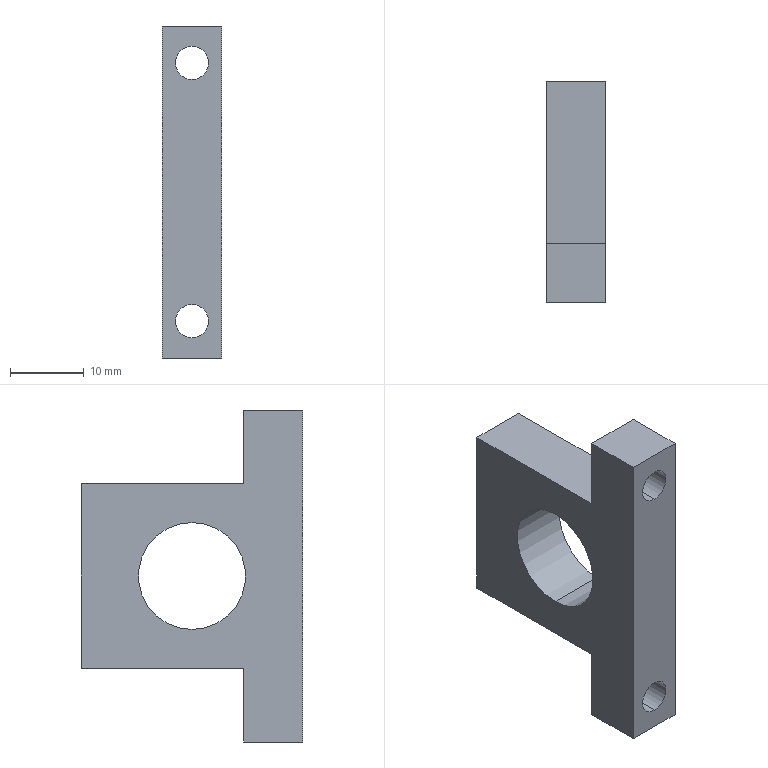Part | STEP file | 04-09 Suction rotary cylinder fixing plate | 1 solid | 16 faces | box 8 x 30 x 45 mm | volume 5704 mm3 | plane 10 | cylinder 6 | commonest cylinder face diameters 4.5 x4 14.5 x2
STEP:
#1=CARTESIAN_POINT('',(0.,0.,0.));
#2=DIRECTION('',(0.,0.,1.));
#3=DIRECTION('',(1.,0.,0.));
#4=AXIS2_PLACEMENT_3D('',#1,#2,#3);
#5=CARTESIAN_POINT('',(4.,0.,19.75));
#6=VERTEX_POINT('',#5);
#7=CARTESIAN_POINT('',(4.,8.,19.75));
#8=VERTEX_POINT('',#7);
#9=CARTESIAN_POINT('',(4.,0.,19.75));
#10=DIRECTION('',(0.,1.,0.));
#11=VECTOR('',#10,1.);
#12=LINE('',#9,#11);
#13=CARTESIAN_POINT('',(4.,0.,17.5));
#14=DIRECTION('',(0.,1.,0.));
#15=DIRECTION('',(0.,0.,1.));
#16=AXIS2_PLACEMENT_3D('',#13,#14,#15);
#17=CYLINDRICAL_SURFACE('',#16,2.25);
#18=CARTESIAN_POINT('',(6.283,0.));
#19=DIRECTION('',(0.,1.));
#20=VECTOR('',#19,1.);
#21=LINE('',#18,#20);
#22=(GEOMETRIC_REPRESENTATION_CONTEXT(2)PARAMETRIC_REPRESENTATION_CONTEXT()REPRESENTATION_CONTEXT('',''));
#23=DEFINITIONAL_REPRESENTATION('',(#21),#22);
#24=PCURVE('',#17,#23);
#25=CARTESIAN_POINT('',(4.,0.,17.5));
#26=DIRECTION('',(0.,1.,0.));
#27=DIRECTION('',(0.,0.,1.));
#28=AXIS2_PLACEMENT_3D('',#25,#26,#27);
#29=CYLINDRICAL_SURFACE('',#28,2.25);
#30=CARTESIAN_POINT('',(0.,0.));
#31=DIRECTION('',(0.,1.));
#32=VECTOR('',#31,1.);
#33=LINE('',#30,#32);
#34=(GEOMETRIC_REPRESENTATION_CONTEXT(2)PARAMETRIC_REPRESENTATION_CONTEXT()REPRESENTATION_CONTEXT('',''));
#35=DEFINITIONAL_REPRESENTATION('',(#33),#34);
#36=PCURVE('',#29,#35);
#37=SURFACE_CURVE('',#12,(#24,#36),.PCURVE_S1.);
#38=EDGE_CURVE('',#6,#8,#37,.T.);
#39=ORIENTED_EDGE('',*,*,#38,.T.);
#40=CARTESIAN_POINT('',(4.,8.,15.25));
#41=VERTEX_POINT('',#40);
#42=CARTESIAN_POINT('',(4.,8.,17.5));
#43=DIRECTION('',(0.,1.,0.));
#44=DIRECTION('',(0.,0.,1.));
#45=AXIS2_PLACEMENT_3D('',#42,#43,#44);
#46=CIRCLE('',#45,2.25);
#47=CARTESIAN_POINT('',(0.,8.));
#48=DIRECTION('',(1.,0.));
#49=VECTOR('',#48,1.);
#50=LINE('',#47,#49);
#51=(GEOMETRIC_REPRESENTATION_CONTEXT(2)PARAMETRIC_REPRESENTATION_CONTEXT()REPRESENTATION_CONTEXT('',''));
#52=DEFINITIONAL_REPRESENTATION('',(#50),#51);
#53=PCURVE('',#17,#52);
#54=CARTESIAN_POINT('',(0.,8.,22.5));
#55=DIRECTION('',(0.,-1.,0.));
#56=DIRECTION('',(0.,0.,-1.));
#57=AXIS2_PLACEMENT_3D('',#54,#55,#56);
#58=PLANE('',#57);
#59=CARTESIAN_POINT('',(2.75,4.));
#60=CARTESIAN_POINT('',(2.75,7.897));
#61=CARTESIAN_POINT('',(6.125,5.949));
#62=CARTESIAN_POINT('',(9.5,4.));
#63=CARTESIAN_POINT('',(6.125,2.051));
#64=CARTESIAN_POINT('',(2.75,0.1029));
#65=CARTESIAN_POINT('',(2.75,4.));
#66=(BOUNDED_CURVE()B_SPLINE_CURVE(2,(#59,#60,#61,#62,#63,#64,#65),.UNSPECIFIED.,.T.,.F.)B_SPLINE_CURVE_WITH_KNOTS((1,2,2,2,2,1),(-2.094,0.,2.094,4.189,6.283,8.378),.UNSPECIFIED.)CURVE()GEOMETRIC_REPRESENTATION_ITEM()RATIONAL_B_SPLINE_CURVE((1.,0.5,1.,0.5,1.,0.5,1.))REPRESENTATION_ITEM(''));
#67=(GEOMETRIC_REPRESENTATION_CONTEXT(2)PARAMETRIC_REPRESENTATION_CONTEXT()REPRESENTATION_CONTEXT('',''));
#68=DEFINITIONAL_REPRESENTATION('',(#66),#67);
#69=PCURVE('',#58,#68);
#70=SURFACE_CURVE('',#46,(#53,#69),.PCURVE_S1.);
#71=EDGE_CURVE('',#41,#8,#70,.T.);
#72=ORIENTED_EDGE('',*,*,#71,.F.);
#73=CARTESIAN_POINT('',(4.,0.,15.25));
#74=VERTEX_POINT('',#73);
#75=CARTESIAN_POINT('',(4.,0.,15.25));
#76=DIRECTION('',(0.,1.,0.));
#77=VECTOR('',#76,1.);
#78=LINE('',#75,#77);
#79=CARTESIAN_POINT('',(3.142,0.));
#80=DIRECTION('',(0.,1.));
#81=VECTOR('',#80,1.);
#82=LINE('',#79,#81);
#83=(GEOMETRIC_REPRESENTATION_CONTEXT(2)PARAMETRIC_REPRESENTATION_CONTEXT()REPRESENTATION_CONTEXT('',''));
#84=DEFINITIONAL_REPRESENTATION('',(#82),#83);
#85=PCURVE('',#17,#84);
#86=CARTESIAN_POINT('',(3.142,0.));
#87=DIRECTION('',(0.,1.));
#88=VECTOR('',#87,1.);
#89=LINE('',#86,#88);
#90=(GEOMETRIC_REPRESENTATION_CONTEXT(2)PARAMETRIC_REPRESENTATION_CONTEXT()REPRESENTATION_CONTEXT('',''));
#91=DEFINITIONAL_REPRESENTATION('',(#89),#90);
#92=PCURVE('',#29,#91);
#93=SURFACE_CURVE('',#78,(#85,#92),.PCURVE_S1.);
#94=EDGE_CURVE('',#74,#41,#93,.T.);
#95=ORIENTED_EDGE('',*,*,#94,.F.);
#96=CARTESIAN_POINT('',(4.,0.,17.5));
#97=DIRECTION('',(0.,-1.,0.));
#98=DIRECTION('',(0.,0.,1.));
#99=AXIS2_PLACEMENT_3D('',#96,#97,#98);
#100=CIRCLE('',#99,2.25);
#101=CARTESIAN_POINT('',(6.283,0.));
#102=DIRECTION('',(-1.,0.));
#103=VECTOR('',#102,1.);
#104=LINE('',#101,#103);
#105=(GEOMETRIC_REPRESENTATION_CONTEXT(2)PARAMETRIC_REPRESENTATION_CONTEXT()REPRESENTATION_CONTEXT('',''));
#106=DEFINITIONAL_REPRESENTATION('',(#104),#105);
#107=PCURVE('',#17,#106);
#108=CARTESIAN_POINT('',(0.,0.,-22.5));
#109=DIRECTION('',(0.,1.,0.));
#110=DIRECTION('',(0.,0.,1.));
#111=AXIS2_PLACEMENT_3D('',#108,#109,#110);
#112=PLANE('',#111);
#113=CARTESIAN_POINT('',(42.25,4.));
#114=CARTESIAN_POINT('',(42.25,0.1029));
#115=CARTESIAN_POINT('',(38.875,2.051));
#116=CARTESIAN_POINT('',(35.5,4.));
#117=CARTESIAN_POINT('',(38.875,5.949));
#118=CARTESIAN_POINT('',(42.25,7.897));
#119=CARTESIAN_POINT('',(42.25,4.));
#120=(BOUNDED_CURVE()B_SPLINE_CURVE(2,(#113,#114,#115,#116,#117,#118,#119),.UNSPECIFIED.,.T.,.F.)B_SPLINE_CURVE_WITH_KNOTS((1,2,2,2,2,1),(-2.094,0.,2.094,4.189,6.283,8.378),.UNSPECIFIED.)CURVE()GEOMETRIC_REPRESENTATION_ITEM()RATIONAL_B_SPLINE_CURVE((1.,0.5,1.,0.5,1.,0.5,1.))REPRESENTATION_ITEM(''));
#121=(GEOMETRIC_REPRESENTATION_CONTEXT(2)PARAMETRIC_REPRESENTATION_CONTEXT()REPRESENTATION_CONTEXT('',''));
#122=DEFINITIONAL_REPRESENTATION('',(#120),#121);
#123=PCURVE('',#112,#122);
#124=SURFACE_CURVE('',#100,(#107,#123),.PCURVE_S1.);
#125=EDGE_CURVE('',#6,#74,#124,.T.);
#126=ORIENTED_EDGE('',*,*,#125,.F.);
#127=EDGE_LOOP('',(#39,#72,#95,#126));
#128=FACE_BOUND('',#127,.F.);
#129=ADVANCED_FACE('',(#128),#17,.F.);
#130=CARTESIAN_POINT('',(4.,0.,-15.25));
#131=VERTEX_POINT('',#130);
#132=CARTESIAN_POINT('',(4.,8.,-15.25));
#133=VERTEX_POINT('',#132);
#134=CARTESIAN_POINT('',(4.,0.,-15.25));
#135=DIRECTION('',(0.,1.,0.));
#136=VECTOR('',#135,1.);
#137=LINE('',#134,#136);
#138=CARTESIAN_POINT('',(4.,0.,-17.5));
#139=DIRECTION('',(0.,1.,0.));
#140=DIRECTION('',(0.,0.,1.));
#141=AXIS2_PLACEMENT_3D('',#138,#139,#140);
#142=CYLINDRICAL_SURFACE('',#141,2.25);
#143=CARTESIAN_POINT('',(6.283,0.));
#144=DIRECTION('',(0.,1.));
#145=VECTOR('',#144,1.);
#146=LINE('',#143,#145);
#147=(GEOMETRIC_REPRESENTATION_CONTEXT(2)PARAMETRIC_REPRESENTATION_CONTEXT()REPRESENTATION_CONTEXT('',''));
#148=DEFINITIONAL_REPRESENTATION('',(#146),#147);
#149=PCURVE('',#142,#148);
#150=CARTESIAN_POINT('',(4.,0.,-17.5));
#151=DIRECTION('',(0.,1.,0.));
#152=DIRECTION('',(0.,0.,1.));
#153=AXIS2_PLACEMENT_3D('',#150,#151,#152);
#154=CYLINDRICAL_SURFACE('',#153,2.25);
#155=CARTESIAN_POINT('',(0.,0.));
#156=DIRECTION('',(0.,1.));
#157=VECTOR('',#156,1.);
#158=LINE('',#155,#157);
#159=(GEOMETRIC_REPRESENTATION_CONTEXT(2)PARAMETRIC_REPRESENTATION_CONTEXT()REPRESENTATION_CONTEXT('',''));
#160=DEFINITIONAL_REPRESENTATION('',(#158),#159);
#161=PCURVE('',#154,#160);
#162=SURFACE_CURVE('',#137,(#149,#161),.PCURVE_S1.);
#163=EDGE_CURVE('',#131,#133,#162,.T.);
#164=ORIENTED_EDGE('',*,*,#163,.T.);
#165=CARTESIAN_POINT('',(4.,8.,-19.75));
#166=VERTEX_POINT('',#165);
#167=CARTESIAN_POINT('',(4.,8.,-17.5));
#168=DIRECTION('',(0.,1.,0.));
#169=DIRECTION('',(0.,0.,1.));
#170=AXIS2_PLACEMENT_3D('',#167,#168,#169);
#171=CIRCLE('',#170,2.25);
#172=CARTESIAN_POINT('',(0.,8.));
#173=DIRECTION('',(1.,0.));
#174=VECTOR('',#173,1.);
#175=LINE('',#172,#174);
#176=(GEOMETRIC_REPRESENTATION_CONTEXT(2)PARAMETRIC_REPRESENTATION_CONTEXT()REPRESENTATION_CONTEXT('',''));
#177=DEFINITIONAL_REPRESENTATION('',(#175),#176);
#178=PCURVE('',#142,#177);
#179=CARTESIAN_POINT('',(0.,8.,-12.5));
#180=DIRECTION('',(0.,-1.,0.));
#181=DIRECTION('',(0.,0.,-1.));
#182=AXIS2_PLACEMENT_3D('',#179,#180,#181);
#183=PLANE('',#182);
#184=CARTESIAN_POINT('',(2.75,4.));
#185=CARTESIAN_POINT('',(2.75,7.897));
#186=CARTESIAN_POINT('',(6.125,5.949));
#187=CARTESIAN_POINT('',(9.5,4.));
#188=CARTESIAN_POINT('',(6.125,2.051));
#189=CARTESIAN_POINT('',(2.75,0.1029));
#190=CARTESIAN_POINT('',(2.75,4.));
#191=(BOUNDED_CURVE()B_SPLINE_CURVE(2,(#184,#185,#186,#187,#188,#189,#190),.UNSPECIFIED.,.T.,.F.)B_SPLINE_CURVE_WITH_KNOTS((1,2,2,2,2,1),(-2.094,0.,2.094,4.189,6.283,8.378),.UNSPECIFIED.)CURVE()GEOMETRIC_REPRESENTATION_ITEM()RATIONAL_B_SPLINE_CURVE((1.,0.5,1.,0.5,1.,0.5,1.))REPRESENTATION_ITEM(''));
#192=(GEOMETRIC_REPRESENTATION_CONTEXT(2)PARAMETRIC_REPRESENTATION_CONTEXT()REPRESENTATION_CONTEXT('',''));
#193=DEFINITIONAL_REPRESENTATION('',(#191),#192);
#194=PCURVE('',#183,#193);
#195=SURFACE_CURVE('',#171,(#178,#194),.PCURVE_S1.);
#196=EDGE_CURVE('',#166,#133,#195,.T.);
#197=ORIENTED_EDGE('',*,*,#196,.F.);
#198=CARTESIAN_POINT('',(4.,0.,-19.75));
#199=VERTEX_POINT('',#198);
#200=CARTESIAN_POINT('',(4.,0.,-19.75));
#201=DIRECTION('',(0.,1.,0.));
#202=VECTOR('',#201,1.);
#203=LINE('',#200,#202);
#204=CARTESIAN_POINT('',(3.142,0.));
#205=DIRECTION('',(0.,1.));
#206=VECTOR('',#205,1.);
#207=LINE('',#204,#206);
#208=(GEOMETRIC_REPRESENTATION_CONTEXT(2)PARAMETRIC_REPRESENTATION_CONTEXT()REPRESENTATION_CONTEXT('',''));
#209=DEFINITIONAL_REPRESENTATION('',(#207),#208);
#210=PCURVE('',#142,#209);
#211=CARTESIAN_POINT('',(3.142,0.));
#212=DIRECTION('',(0.,1.));
#213=VECTOR('',#212,1.);
#214=LINE('',#211,#213);
#215=(GEOMETRIC_REPRESENTATION_CONTEXT(2)PARAMETRIC_REPRESENTATION_CONTEXT()REPRESENTATION_CONTEXT('',''));
#216=DEFINITIONAL_REPRESENTATION('',(#214),#215);
#217=PCURVE('',#154,#216);
#218=SURFACE_CURVE('',#203,(#210,#217),.PCURVE_S1.);
#219=EDGE_CURVE('',#199,#166,#218,.T.);
#220=ORIENTED_EDGE('',*,*,#219,.F.);
#221=CARTESIAN_POINT('',(4.,0.,-17.5));
#222=DIRECTION('',(0.,-1.,0.));
#223=DIRECTION('',(0.,0.,1.));
#224=AXIS2_PLACEMENT_3D('',#221,#222,#223);
#225=CIRCLE('',#224,2.25);
#226=CARTESIAN_POINT('',(6.283,0.));
#227=DIRECTION('',(-1.,0.));
#228=VECTOR('',#227,1.);
#229=LINE('',#226,#228);
#230=(GEOMETRIC_REPRESENTATION_CONTEXT(2)PARAMETRIC_REPRESENTATION_CONTEXT()REPRESENTATION_CONTEXT('',''));
#231=DEFINITIONAL_REPRESENTATION('',(#229),#230);
#232=PCURVE('',#142,#231);
#233=CARTESIAN_POINT('',(7.25,4.));
#234=CARTESIAN_POINT('',(7.25,0.1029));
#235=CARTESIAN_POINT('',(3.875,2.051));
#236=CARTESIAN_POINT('',(0.5,4.));
#237=CARTESIAN_POINT('',(3.875,5.949));
#238=CARTESIAN_POINT('',(7.25,7.897));
#239=CARTESIAN_POINT('',(7.25,4.));
#240=(BOUNDED_CURVE()B_SPLINE_CURVE(2,(#233,#234,#235,#236,#237,#238,#239),.UNSPECIFIED.,.T.,.F.)B_SPLINE_CURVE_WITH_KNOTS((1,2,2,2,2,1),(-2.094,0.,2.094,4.189,6.283,8.378),.UNSPECIFIED.)CURVE()GEOMETRIC_REPRESENTATION_ITEM()RATIONAL_B_SPLINE_CURVE((1.,0.5,1.,0.5,1.,0.5,1.))REPRESENTATION_ITEM(''));
#241=(GEOMETRIC_REPRESENTATION_CONTEXT(2)PARAMETRIC_REPRESENTATION_CONTEXT()REPRESENTATION_CONTEXT('',''));
#242=DEFINITIONAL_REPRESENTATION('',(#240),#241);
#243=PCURVE('',#112,#242);
#244=SURFACE_CURVE('',#225,(#232,#243),.PCURVE_S1.);
#245=EDGE_CURVE('',#131,#199,#244,.T.);
#246=ORIENTED_EDGE('',*,*,#245,.F.);
#247=EDGE_LOOP('',(#164,#197,#220,#246));
#248=FACE_BOUND('',#247,.F.);
#249=ADVANCED_FACE('',(#248),#142,.F.);
#250=CARTESIAN_POINT('',(0.,15.,-7.25));
#251=VERTEX_POINT('',#250);
#252=CARTESIAN_POINT('',(8.,15.,-7.25));
#253=VERTEX_POINT('',#252);
#254=CARTESIAN_POINT('',(0.,15.,-7.25));
#255=DIRECTION('',(1.,0.,0.));
#256=VECTOR('',#255,1.);
#257=LINE('',#254,#256);
#258=CARTESIAN_POINT('',(0.,15.,0.));
#259=DIRECTION('',(1.,0.,0.));
#260=DIRECTION('',(0.,0.,-1.));
#261=AXIS2_PLACEMENT_3D('',#258,#259,#260);
#262=CYLINDRICAL_SURFACE('',#261,7.25);
#263=CARTESIAN_POINT('',(6.283,0.));
#264=DIRECTION('',(0.,1.));
#265=VECTOR('',#264,1.);
#266=LINE('',#263,#265);
#267=(GEOMETRIC_REPRESENTATION_CONTEXT(2)PARAMETRIC_REPRESENTATION_CONTEXT()REPRESENTATION_CONTEXT('',''));
#268=DEFINITIONAL_REPRESENTATION('',(#266),#267);
#269=PCURVE('',#262,#268);
#270=CARTESIAN_POINT('',(0.,15.,0.));
#271=DIRECTION('',(1.,0.,0.));
#272=DIRECTION('',(0.,0.,-1.));
#273=AXIS2_PLACEMENT_3D('',#270,#271,#272);
#274=CYLINDRICAL_SURFACE('',#273,7.25);
#275=CARTESIAN_POINT('',(0.,0.));
#276=DIRECTION('',(0.,1.));
#277=VECTOR('',#276,1.);
#278=LINE('',#275,#277);
#279=(GEOMETRIC_REPRESENTATION_CONTEXT(2)PARAMETRIC_REPRESENTATION_CONTEXT()REPRESENTATION_CONTEXT('',''));
#280=DEFINITIONAL_REPRESENTATION('',(#278),#279);
#281=PCURVE('',#274,#280);
#282=SURFACE_CURVE('',#257,(#269,#281),.PCURVE_S1.);
#283=EDGE_CURVE('',#251,#253,#282,.T.);
#284=ORIENTED_EDGE('',*,*,#283,.T.);
#285=CARTESIAN_POINT('',(8.,15.,7.25));
#286=VERTEX_POINT('',#285);
#287=CARTESIAN_POINT('',(8.,15.,0.));
#288=DIRECTION('',(1.,0.,0.));
#289=DIRECTION('',(0.,0.,-1.));
#290=AXIS2_PLACEMENT_3D('',#287,#288,#289);
#291=CIRCLE('',#290,7.25);
#292=CARTESIAN_POINT('',(0.,8.));
#293=DIRECTION('',(1.,0.));
#294=VECTOR('',#293,1.);
#295=LINE('',#292,#294);
#296=(GEOMETRIC_REPRESENTATION_CONTEXT(2)PARAMETRIC_REPRESENTATION_CONTEXT()REPRESENTATION_CONTEXT('',''));
#297=DEFINITIONAL_REPRESENTATION('',(#295),#296);
#298=PCURVE('',#262,#297);
#299=CARTESIAN_POINT('',(8.,0.,-22.5));
#300=DIRECTION('',(-1.,0.,0.));
#301=DIRECTION('',(0.,0.,1.));
#302=AXIS2_PLACEMENT_3D('',#299,#300,#301);
#303=PLANE('',#302);
#304=CARTESIAN_POINT('',(15.25,15.));
#305=CARTESIAN_POINT('',(15.25,27.557));
#306=CARTESIAN_POINT('',(26.125,21.279));
#307=CARTESIAN_POINT('',(37.,15.));
#308=CARTESIAN_POINT('',(26.125,8.721));
#309=CARTESIAN_POINT('',(15.25,2.443));
#310=CARTESIAN_POINT('',(15.25,15.));
#311=(BOUNDED_CURVE()B_SPLINE_CURVE(2,(#304,#305,#306,#307,#308,#309,#310),.UNSPECIFIED.,.T.,.F.)B_SPLINE_CURVE_WITH_KNOTS((1,2,2,2,2,1),(-2.094,0.,2.094,4.189,6.283,8.378),.UNSPECIFIED.)CURVE()GEOMETRIC_REPRESENTATION_ITEM()RATIONAL_B_SPLINE_CURVE((1.,0.5,1.,0.5,1.,0.5,1.))REPRESENTATION_ITEM(''));
#312=(GEOMETRIC_REPRESENTATION_CONTEXT(2)PARAMETRIC_REPRESENTATION_CONTEXT()REPRESENTATION_CONTEXT('',''));
#313=DEFINITIONAL_REPRESENTATION('',(#311),#312);
#314=PCURVE('',#303,#313);
#315=SURFACE_CURVE('',#291,(#298,#314),.PCURVE_S1.);
#316=EDGE_CURVE('',#286,#253,#315,.T.);
#317=ORIENTED_EDGE('',*,*,#316,.F.);
#318=CARTESIAN_POINT('',(0.,15.,7.25));
#319=VERTEX_POINT('',#318);
#320=CARTESIAN_POINT('',(0.,15.,7.25));
#321=DIRECTION('',(1.,0.,0.));
#322=VECTOR('',#321,1.);
#323=LINE('',#320,#322);
#324=CARTESIAN_POINT('',(3.142,0.));
#325=DIRECTION('',(0.,1.));
#326=VECTOR('',#325,1.);
#327=LINE('',#324,#326);
#328=(GEOMETRIC_REPRESENTATION_CONTEXT(2)PARAMETRIC_REPRESENTATION_CONTEXT()REPRESENTATION_CONTEXT('',''));
#329=DEFINITIONAL_REPRESENTATION('',(#327),#328);
#330=PCURVE('',#262,#329);
#331=CARTESIAN_POINT('',(3.142,0.));
#332=DIRECTION('',(0.,1.));
#333=VECTOR('',#332,1.);
#334=LINE('',#331,#333);
#335=(GEOMETRIC_REPRESENTATION_CONTEXT(2)PARAMETRIC_REPRESENTATION_CONTEXT()REPRESENTATION_CONTEXT('',''));
#336=DEFINITIONAL_REPRESENTATION('',(#334),#335);
#337=PCURVE('',#274,#336);
#338=SURFACE_CURVE('',#323,(#330,#337),.PCURVE_S1.);
#339=EDGE_CURVE('',#319,#286,#338,.T.);
#340=ORIENTED_EDGE('',*,*,#339,.F.);
#341=CARTESIAN_POINT('',(0.,15.,0.));
#342=DIRECTION('',(1.,0.,0.));
#343=DIRECTION('',(0.,0.,-1.));
#344=AXIS2_PLACEMENT_3D('',#341,#342,#343);
#345=CIRCLE('',#344,7.25);
#346=CARTESIAN_POINT('',(0.,0.));
#347=DIRECTION('',(1.,0.));
#348=VECTOR('',#347,1.);
#349=LINE('',#346,#348);
#350=(GEOMETRIC_REPRESENTATION_CONTEXT(2)PARAMETRIC_REPRESENTATION_CONTEXT()REPRESENTATION_CONTEXT('',''));
#351=DEFINITIONAL_REPRESENTATION('',(#349),#350);
#352=PCURVE('',#262,#351);
#353=CARTESIAN_POINT('',(0.,0.,-22.5));
#354=DIRECTION('',(-1.,0.,0.));
#355=DIRECTION('',(0.,0.,1.));
#356=AXIS2_PLACEMENT_3D('',#353,#354,#355);
#357=PLANE('',#356);
#358=CARTESIAN_POINT('',(15.25,15.));
#359=CARTESIAN_POINT('',(15.25,27.557));
#360=CARTESIAN_POINT('',(26.125,21.279));
#361=CARTESIAN_POINT('',(37.,15.));
#362=CARTESIAN_POINT('',(26.125,8.721));
#363=CARTESIAN_POINT('',(15.25,2.443));
#364=CARTESIAN_POINT('',(15.25,15.));
#365=(BOUNDED_CURVE()B_SPLINE_CURVE(2,(#358,#359,#360,#361,#362,#363,#364),.UNSPECIFIED.,.T.,.F.)B_SPLINE_CURVE_WITH_KNOTS((1,2,2,2,2,1),(-2.094,0.,2.094,4.189,6.283,8.378),.UNSPECIFIED.)CURVE()GEOMETRIC_REPRESENTATION_ITEM()RATIONAL_B_SPLINE_CURVE((1.,0.5,1.,0.5,1.,0.5,1.))REPRESENTATION_ITEM(''));
#366=(GEOMETRIC_REPRESENTATION_CONTEXT(2)PARAMETRIC_REPRESENTATION_CONTEXT()REPRESENTATION_CONTEXT('',''));
#367=DEFINITIONAL_REPRESENTATION('',(#365),#366);
#368=PCURVE('',#357,#367);
#369=SURFACE_CURVE('',#345,(#352,#368),.PCURVE_S1.);
#370=EDGE_CURVE('',#319,#251,#369,.T.);
#371=ORIENTED_EDGE('',*,*,#370,.T.);
#372=EDGE_LOOP('',(#284,#317,#340,#371));
#373=FACE_BOUND('',#372,.F.);
#374=ADVANCED_FACE('',(#373),#262,.F.);
#375=CARTESIAN_POINT('',(4.,8.,17.5));
#376=DIRECTION('',(0.,1.,0.));
#377=DIRECTION('',(0.,0.,1.));
#378=AXIS2_PLACEMENT_3D('',#375,#376,#377);
#379=CIRCLE('',#378,2.25);
#380=CARTESIAN_POINT('',(0.,8.));
#381=DIRECTION('',(1.,0.));
#382=VECTOR('',#381,1.);
#383=LINE('',#380,#382);
#384=(GEOMETRIC_REPRESENTATION_CONTEXT(2)PARAMETRIC_REPRESENTATION_CONTEXT()REPRESENTATION_CONTEXT('',''));
#385=DEFINITIONAL_REPRESENTATION('',(#383),#384);
#386=PCURVE('',#29,#385);
#387=CARTESIAN_POINT('',(2.75,4.));
#388=CARTESIAN_POINT('',(2.75,7.897));
#389=CARTESIAN_POINT('',(6.125,5.949));
#390=CARTESIAN_POINT('',(9.5,4.));
#391=CARTESIAN_POINT('',(6.125,2.051));
#392=CARTESIAN_POINT('',(2.75,0.1029));
#393=CARTESIAN_POINT('',(2.75,4.));
#394=(BOUNDED_CURVE()B_SPLINE_CURVE(2,(#387,#388,#389,#390,#391,#392,#393),.UNSPECIFIED.,.T.,.F.)B_SPLINE_CURVE_WITH_KNOTS((1,2,2,2,2,1),(-2.094,0.,2.094,4.189,6.283,8.378),.UNSPECIFIED.)CURVE()GEOMETRIC_REPRESENTATION_ITEM()RATIONAL_B_SPLINE_CURVE((1.,0.5,1.,0.5,1.,0.5,1.))REPRESENTATION_ITEM(''));
#395=(GEOMETRIC_REPRESENTATION_CONTEXT(2)PARAMETRIC_REPRESENTATION_CONTEXT()REPRESENTATION_CONTEXT('',''));
#396=DEFINITIONAL_REPRESENTATION('',(#394),#395);
#397=PCURVE('',#58,#396);
#398=SURFACE_CURVE('',#379,(#386,#397),.PCURVE_S1.);
#399=EDGE_CURVE('',#8,#41,#398,.T.);
#400=ORIENTED_EDGE('',*,*,#399,.F.);
#401=ORIENTED_EDGE('',*,*,#38,.F.);
#402=CARTESIAN_POINT('',(4.,0.,17.5));
#403=DIRECTION('',(0.,-1.,0.));
#404=DIRECTION('',(0.,0.,1.));
#405=AXIS2_PLACEMENT_3D('',#402,#403,#404);
#406=CIRCLE('',#405,2.25);
#407=CARTESIAN_POINT('',(6.283,0.));
#408=DIRECTION('',(-1.,0.));
#409=VECTOR('',#408,1.);
#410=LINE('',#407,#409);
#411=(GEOMETRIC_REPRESENTATION_CONTEXT(2)PARAMETRIC_REPRESENTATION_CONTEXT()REPRESENTATION_CONTEXT('',''));
#412=DEFINITIONAL_REPRESENTATION('',(#410),#411);
#413=PCURVE('',#29,#412);
#414=CARTESIAN_POINT('',(42.25,4.));
#415=CARTESIAN_POINT('',(42.25,0.1029));
#416=CARTESIAN_POINT('',(38.875,2.051));
#417=CARTESIAN_POINT('',(35.5,4.));
#418=CARTESIAN_POINT('',(38.875,5.949));
#419=CARTESIAN_POINT('',(42.25,7.897));
#420=CARTESIAN_POINT('',(42.25,4.));
#421=(BOUNDED_CURVE()B_SPLINE_CURVE(2,(#414,#415,#416,#417,#418,#419,#420),.UNSPECIFIED.,.T.,.F.)B_SPLINE_CURVE_WITH_KNOTS((1,2,2,2,2,1),(-2.094,0.,2.094,4.189,6.283,8.378),.UNSPECIFIED.)CURVE()GEOMETRIC_REPRESENTATION_ITEM()RATIONAL_B_SPLINE_CURVE((1.,0.5,1.,0.5,1.,0.5,1.))REPRESENTATION_ITEM(''));
#422=(GEOMETRIC_REPRESENTATION_CONTEXT(2)PARAMETRIC_REPRESENTATION_CONTEXT()REPRESENTATION_CONTEXT('',''));
#423=DEFINITIONAL_REPRESENTATION('',(#421),#422);
#424=PCURVE('',#112,#423);
#425=SURFACE_CURVE('',#406,(#413,#424),.PCURVE_S1.);
#426=EDGE_CURVE('',#74,#6,#425,.T.);
#427=ORIENTED_EDGE('',*,*,#426,.F.);
#428=ORIENTED_EDGE('',*,*,#94,.T.);
#429=EDGE_LOOP('',(#400,#401,#427,#428));
#430=FACE_BOUND('',#429,.F.);
#431=ADVANCED_FACE('',(#430),#29,.F.);
#432=ORIENTED_EDGE('',*,*,#399,.F.);
#433=ORIENTED_EDGE('',*,*,#71,.F.);
#434=EDGE_LOOP('',(#432,#433));
#435=FACE_BOUND('',#434,.T.);
#436=CARTESIAN_POINT('',(8.,8.,22.5));
#437=VERTEX_POINT('',#436);
#438=CARTESIAN_POINT('',(0.,8.,22.5));
#439=VERTEX_POINT('',#438);
#440=CARTESIAN_POINT('',(4.,8.,22.5));
#441=DIRECTION('',(-1.,0.,0.));
#442=VECTOR('',#441,1.);
#443=LINE('',#440,#442);
#444=CARTESIAN_POINT('',(0.,4.));
#445=DIRECTION('',(0.,-1.));
#446=VECTOR('',#445,1.);
#447=LINE('',#444,#446);
#448=(GEOMETRIC_REPRESENTATION_CONTEXT(2)PARAMETRIC_REPRESENTATION_CONTEXT()REPRESENTATION_CONTEXT('',''));
#449=DEFINITIONAL_REPRESENTATION('',(#447),#448);
#450=PCURVE('',#58,#449);
#451=CARTESIAN_POINT('',(8.,0.,22.5));
#452=DIRECTION('',(0.,0.,-1.));
#453=DIRECTION('',(-1.,0.,0.));
#454=AXIS2_PLACEMENT_3D('',#451,#452,#453);
#455=PLANE('',#454);
#456=CARTESIAN_POINT('',(4.,8.));
#457=DIRECTION('',(1.,0.));
#458=VECTOR('',#457,1.);
#459=LINE('',#456,#458);
#460=(GEOMETRIC_REPRESENTATION_CONTEXT(2)PARAMETRIC_REPRESENTATION_CONTEXT()REPRESENTATION_CONTEXT('',''));
#461=DEFINITIONAL_REPRESENTATION('',(#459),#460);
#462=PCURVE('',#455,#461);
#463=SURFACE_CURVE('',#443,(#450,#462),.PCURVE_S1.);
#464=EDGE_CURVE('',#437,#439,#463,.T.);
#465=ORIENTED_EDGE('',*,*,#464,.F.);
#466=CARTESIAN_POINT('',(8.,8.,12.5));
#467=VERTEX_POINT('',#466);
#468=CARTESIAN_POINT('',(8.,8.,17.5));
#469=DIRECTION('',(0.,0.,1.));
#470=VECTOR('',#469,1.);
#471=LINE('',#468,#470);
#472=CARTESIAN_POINT('',(5.,8.));
#473=DIRECTION('',(-1.,0.));
#474=VECTOR('',#473,1.);
#475=LINE('',#472,#474);
#476=(GEOMETRIC_REPRESENTATION_CONTEXT(2)PARAMETRIC_REPRESENTATION_CONTEXT()REPRESENTATION_CONTEXT('',''));
#477=DEFINITIONAL_REPRESENTATION('',(#475),#476);
#478=PCURVE('',#58,#477);
#479=CARTESIAN_POINT('',(40.,8.));
#480=DIRECTION('',(1.,0.));
#481=VECTOR('',#480,1.);
#482=LINE('',#479,#481);
#483=(GEOMETRIC_REPRESENTATION_CONTEXT(2)PARAMETRIC_REPRESENTATION_CONTEXT()REPRESENTATION_CONTEXT('',''));
#484=DEFINITIONAL_REPRESENTATION('',(#482),#483);
#485=PCURVE('',#303,#484);
#486=SURFACE_CURVE('',#471,(#478,#485),.PCURVE_S1.);
#487=EDGE_CURVE('',#467,#437,#486,.T.);
#488=ORIENTED_EDGE('',*,*,#487,.F.);
#489=CARTESIAN_POINT('',(0.,8.,12.5));
#490=VERTEX_POINT('',#489);
#491=CARTESIAN_POINT('',(4.,8.,12.5));
#492=DIRECTION('',(1.,0.,0.));
#493=VECTOR('',#492,1.);
#494=LINE('',#491,#493);
#495=CARTESIAN_POINT('',(10.,4.));
#496=DIRECTION('',(0.,1.));
#497=VECTOR('',#496,1.);
#498=LINE('',#495,#497);
#499=(GEOMETRIC_REPRESENTATION_CONTEXT(2)PARAMETRIC_REPRESENTATION_CONTEXT()REPRESENTATION_CONTEXT('',''));
#500=DEFINITIONAL_REPRESENTATION('',(#498),#499);
#501=PCURVE('',#58,#500);
#502=CARTESIAN_POINT('',(0.,8.,12.5));
#503=DIRECTION('',(0.,0.,-1.));
#504=DIRECTION('',(0.,1.,0.));
#505=AXIS2_PLACEMENT_3D('',#502,#503,#504);
#506=PLANE('',#505);
#507=CARTESIAN_POINT('',(0.,4.));
#508=DIRECTION('',(0.,1.));
#509=VECTOR('',#508,1.);
#510=LINE('',#507,#509);
#511=(GEOMETRIC_REPRESENTATION_CONTEXT(2)PARAMETRIC_REPRESENTATION_CONTEXT()REPRESENTATION_CONTEXT('',''));
#512=DEFINITIONAL_REPRESENTATION('',(#510),#511);
#513=PCURVE('',#506,#512);
#514=SURFACE_CURVE('',#494,(#501,#513),.PCURVE_S1.);
#515=EDGE_CURVE('',#490,#467,#514,.T.);
#516=ORIENTED_EDGE('',*,*,#515,.F.);
#517=CARTESIAN_POINT('',(0.,8.,17.5));
#518=DIRECTION('',(0.,0.,-1.));
#519=VECTOR('',#518,1.);
#520=LINE('',#517,#519);
#521=CARTESIAN_POINT('',(5.,0.));
#522=DIRECTION('',(1.,0.));
#523=VECTOR('',#522,1.);
#524=LINE('',#521,#523);
#525=(GEOMETRIC_REPRESENTATION_CONTEXT(2)PARAMETRIC_REPRESENTATION_CONTEXT()REPRESENTATION_CONTEXT('',''));
#526=DEFINITIONAL_REPRESENTATION('',(#524),#525);
#527=PCURVE('',#58,#526);
#528=CARTESIAN_POINT('',(40.,8.));
#529=DIRECTION('',(-1.,0.));
#530=VECTOR('',#529,1.);
#531=LINE('',#528,#530);
#532=(GEOMETRIC_REPRESENTATION_CONTEXT(2)PARAMETRIC_REPRESENTATION_CONTEXT()REPRESENTATION_CONTEXT('',''));
#533=DEFINITIONAL_REPRESENTATION('',(#531),#532);
#534=PCURVE('',#357,#533);
#535=SURFACE_CURVE('',#520,(#527,#534),.PCURVE_S1.);
#536=EDGE_CURVE('',#439,#490,#535,.T.);
#537=ORIENTED_EDGE('',*,*,#536,.F.);
#538=EDGE_LOOP('',(#465,#488,#516,#537));
#539=FACE_BOUND('',#538,.T.);
#540=ADVANCED_FACE('',(#435,#539),#58,.F.);
#541=ORIENTED_EDGE('',*,*,#245,.F.);
#542=CARTESIAN_POINT('',(4.,0.,-17.5));
#543=DIRECTION('',(0.,-1.,0.));
#544=DIRECTION('',(0.,0.,1.));
#545=AXIS2_PLACEMENT_3D('',#542,#543,#544);
#546=CIRCLE('',#545,2.25);
#547=CARTESIAN_POINT('',(7.25,4.));
#548=CARTESIAN_POINT('',(7.25,0.1029));
#549=CARTESIAN_POINT('',(3.875,2.051));
#550=CARTESIAN_POINT('',(0.5,4.));
#551=CARTESIAN_POINT('',(3.875,5.949));
#552=CARTESIAN_POINT('',(7.25,7.897));
#553=CARTESIAN_POINT('',(7.25,4.));
#554=(BOUNDED_CURVE()B_SPLINE_CURVE(2,(#547,#548,#549,#550,#551,#552,#553),.UNSPECIFIED.,.T.,.F.)B_SPLINE_CURVE_WITH_KNOTS((1,2,2,2,2,1),(-2.094,0.,2.094,4.189,6.283,8.378),.UNSPECIFIED.)CURVE()GEOMETRIC_REPRESENTATION_ITEM()RATIONAL_B_SPLINE_CURVE((1.,0.5,1.,0.5,1.,0.5,1.))REPRESENTATION_ITEM(''));
#555=(GEOMETRIC_REPRESENTATION_CONTEXT(2)PARAMETRIC_REPRESENTATION_CONTEXT()REPRESENTATION_CONTEXT('',''));
#556=DEFINITIONAL_REPRESENTATION('',(#554),#555);
#557=PCURVE('',#112,#556);
#558=CARTESIAN_POINT('',(6.283,0.));
#559=DIRECTION('',(-1.,0.));
#560=VECTOR('',#559,1.);
#561=LINE('',#558,#560);
#562=(GEOMETRIC_REPRESENTATION_CONTEXT(2)PARAMETRIC_REPRESENTATION_CONTEXT()REPRESENTATION_CONTEXT('',''));
#563=DEFINITIONAL_REPRESENTATION('',(#561),#562);
#564=PCURVE('',#154,#563);
#565=SURFACE_CURVE('',#546,(#557,#564),.PCURVE_S1.);
#566=EDGE_CURVE('',#199,#131,#565,.T.);
#567=ORIENTED_EDGE('',*,*,#566,.F.);
#568=EDGE_LOOP('',(#541,#567));
#569=FACE_BOUND('',#568,.T.);
#570=ORIENTED_EDGE('',*,*,#125,.F.);
#571=ORIENTED_EDGE('',*,*,#426,.F.);
#572=EDGE_LOOP('',(#570,#571));
#573=FACE_BOUND('',#572,.T.);
#574=CARTESIAN_POINT('',(8.,0.,-22.5));
#575=VERTEX_POINT('',#574);
#576=CARTESIAN_POINT('',(0.,0.,-22.5));
#577=VERTEX_POINT('',#576);
#578=CARTESIAN_POINT('',(4.,0.,-22.5));
#579=DIRECTION('',(-1.,0.,0.));
#580=VECTOR('',#579,1.);
#581=LINE('',#578,#580);
#582=CARTESIAN_POINT('',(0.,4.));
#583=DIRECTION('',(0.,-1.));
#584=VECTOR('',#583,1.);
#585=LINE('',#582,#584);
#586=(GEOMETRIC_REPRESENTATION_CONTEXT(2)PARAMETRIC_REPRESENTATION_CONTEXT()REPRESENTATION_CONTEXT('',''));
#587=DEFINITIONAL_REPRESENTATION('',(#585),#586);
#588=PCURVE('',#112,#587);
#589=CARTESIAN_POINT('',(0.,0.,-22.5));
#590=DIRECTION('',(0.,0.,1.));
#591=DIRECTION('',(1.,0.,0.));
#592=AXIS2_PLACEMENT_3D('',#589,#590,#591);
#593=PLANE('',#592);
#594=CARTESIAN_POINT('',(4.,0.));
#595=DIRECTION('',(-1.,0.));
#596=VECTOR('',#595,1.);
#597=LINE('',#594,#596);
#598=(GEOMETRIC_REPRESENTATION_CONTEXT(2)PARAMETRIC_REPRESENTATION_CONTEXT()REPRESENTATION_CONTEXT('',''));
#599=DEFINITIONAL_REPRESENTATION('',(#597),#598);
#600=PCURVE('',#593,#599);
#601=SURFACE_CURVE('',#581,(#588,#600),.PCURVE_S1.);
#602=EDGE_CURVE('',#575,#577,#601,.T.);
#603=ORIENTED_EDGE('',*,*,#602,.F.);
#604=CARTESIAN_POINT('',(8.,0.,22.5));
#605=VERTEX_POINT('',#604);
#606=CARTESIAN_POINT('',(8.,0.,0.));
#607=DIRECTION('',(0.,0.,-1.));
#608=VECTOR('',#607,1.);
#609=LINE('',#606,#608);
#610=CARTESIAN_POINT('',(22.5,8.));
#611=DIRECTION('',(-1.,0.));
#612=VECTOR('',#611,1.);
#613=LINE('',#610,#612);
#614=(GEOMETRIC_REPRESENTATION_CONTEXT(2)PARAMETRIC_REPRESENTATION_CONTEXT()REPRESENTATION_CONTEXT('',''));
#615=DEFINITIONAL_REPRESENTATION('',(#613),#614);
#616=PCURVE('',#112,#615);
#617=CARTESIAN_POINT('',(22.5,0.));
#618=DIRECTION('',(-1.,0.));
#619=VECTOR('',#618,1.);
#620=LINE('',#617,#619);
#621=(GEOMETRIC_REPRESENTATION_CONTEXT(2)PARAMETRIC_REPRESENTATION_CONTEXT()REPRESENTATION_CONTEXT('',''));
#622=DEFINITIONAL_REPRESENTATION('',(#620),#621);
#623=PCURVE('',#303,#622);
#624=SURFACE_CURVE('',#609,(#616,#623),.PCURVE_S1.);
#625=EDGE_CURVE('',#605,#575,#624,.T.);
#626=ORIENTED_EDGE('',*,*,#625,.F.);
#627=CARTESIAN_POINT('',(0.,0.,22.5));
#628=VERTEX_POINT('',#627);
#629=CARTESIAN_POINT('',(4.,0.,22.5));
#630=DIRECTION('',(1.,0.,0.));
#631=VECTOR('',#630,1.);
#632=LINE('',#629,#631);
#633=CARTESIAN_POINT('',(45.,4.));
#634=DIRECTION('',(0.,1.));
#635=VECTOR('',#634,1.);
#636=LINE('',#633,#635);
#637=(GEOMETRIC_REPRESENTATION_CONTEXT(2)PARAMETRIC_REPRESENTATION_CONTEXT()REPRESENTATION_CONTEXT('',''));
#638=DEFINITIONAL_REPRESENTATION('',(#636),#637);
#639=PCURVE('',#112,#638);
#640=CARTESIAN_POINT('',(4.,0.));
#641=DIRECTION('',(-1.,0.));
#642=VECTOR('',#641,1.);
#643=LINE('',#640,#642);
#644=(GEOMETRIC_REPRESENTATION_CONTEXT(2)PARAMETRIC_REPRESENTATION_CONTEXT()REPRESENTATION_CONTEXT('',''));
#645=DEFINITIONAL_REPRESENTATION('',(#643),#644);
#646=PCURVE('',#455,#645);
#647=SURFACE_CURVE('',#632,(#639,#646),.PCURVE_S1.);
#648=EDGE_CURVE('',#628,#605,#647,.T.);
#649=ORIENTED_EDGE('',*,*,#648,.F.);
#650=CARTESIAN_POINT('',(0.,0.,0.));
#651=DIRECTION('',(0.,0.,1.));
#652=VECTOR('',#651,1.);
#653=LINE('',#650,#652);
#654=CARTESIAN_POINT('',(22.5,0.));
#655=DIRECTION('',(1.,0.));
#656=VECTOR('',#655,1.);
#657=LINE('',#654,#656);
#658=(GEOMETRIC_REPRESENTATION_CONTEXT(2)PARAMETRIC_REPRESENTATION_CONTEXT()REPRESENTATION_CONTEXT('',''));
#659=DEFINITIONAL_REPRESENTATION('',(#657),#658);
#660=PCURVE('',#112,#659);
#661=CARTESIAN_POINT('',(22.5,0.));
#662=DIRECTION('',(1.,0.));
#663=VECTOR('',#662,1.);
#664=LINE('',#661,#663);
#665=(GEOMETRIC_REPRESENTATION_CONTEXT(2)PARAMETRIC_REPRESENTATION_CONTEXT()REPRESENTATION_CONTEXT('',''));
#666=DEFINITIONAL_REPRESENTATION('',(#664),#665);
#667=PCURVE('',#357,#666);
#668=SURFACE_CURVE('',#653,(#660,#667),.PCURVE_S1.);
#669=EDGE_CURVE('',#577,#628,#668,.T.);
#670=ORIENTED_EDGE('',*,*,#669,.F.);
#671=EDGE_LOOP('',(#603,#626,#649,#670));
#672=FACE_BOUND('',#671,.T.);
#673=ADVANCED_FACE('',(#569,#573,#672),#112,.F.);
#674=CARTESIAN_POINT('',(0.,15.,0.));
#675=DIRECTION('',(1.,0.,0.));
#676=DIRECTION('',(0.,0.,-1.));
#677=AXIS2_PLACEMENT_3D('',#674,#675,#676);
#678=CIRCLE('',#677,7.25);
#679=CARTESIAN_POINT('',(15.25,15.));
#680=CARTESIAN_POINT('',(15.25,27.557));
#681=CARTESIAN_POINT('',(26.125,21.279));
#682=CARTESIAN_POINT('',(37.,15.));
#683=CARTESIAN_POINT('',(26.125,8.721));
#684=CARTESIAN_POINT('',(15.25,2.443));
#685=CARTESIAN_POINT('',(15.25,15.));
#686=(BOUNDED_CURVE()B_SPLINE_CURVE(2,(#679,#680,#681,#682,#683,#684,#685),.UNSPECIFIED.,.T.,.F.)B_SPLINE_CURVE_WITH_KNOTS((1,2,2,2,2,1),(-2.094,0.,2.094,4.189,6.283,8.378),.UNSPECIFIED.)CURVE()GEOMETRIC_REPRESENTATION_ITEM()RATIONAL_B_SPLINE_CURVE((1.,0.5,1.,0.5,1.,0.5,1.))REPRESENTATION_ITEM(''));
#687=(GEOMETRIC_REPRESENTATION_CONTEXT(2)PARAMETRIC_REPRESENTATION_CONTEXT()REPRESENTATION_CONTEXT('',''));
#688=DEFINITIONAL_REPRESENTATION('',(#686),#687);
#689=PCURVE('',#357,#688);
#690=CARTESIAN_POINT('',(0.,0.));
#691=DIRECTION('',(1.,0.));
#692=VECTOR('',#691,1.);
#693=LINE('',#690,#692);
#694=(GEOMETRIC_REPRESENTATION_CONTEXT(2)PARAMETRIC_REPRESENTATION_CONTEXT()REPRESENTATION_CONTEXT('',''));
#695=DEFINITIONAL_REPRESENTATION('',(#693),#694);
#696=PCURVE('',#274,#695);
#697=SURFACE_CURVE('',#678,(#689,#696),.PCURVE_S1.);
#698=EDGE_CURVE('',#251,#319,#697,.T.);
#699=ORIENTED_EDGE('',*,*,#698,.T.);
#700=ORIENTED_EDGE('',*,*,#370,.T.);
#701=EDGE_LOOP('',(#699,#700));
#702=FACE_BOUND('',#701,.T.);
#703=CARTESIAN_POINT('',(0.,8.,-22.5));
#704=VERTEX_POINT('',#703);
#705=CARTESIAN_POINT('',(0.,15.,-22.5));
#706=DIRECTION('',(0.,-1.,0.));
#707=VECTOR('',#706,1.);
#708=LINE('',#705,#707);
#709=CARTESIAN_POINT('',(0.,15.));
#710=DIRECTION('',(0.,-1.));
#711=VECTOR('',#710,1.);
#712=LINE('',#709,#711);
#713=(GEOMETRIC_REPRESENTATION_CONTEXT(2)PARAMETRIC_REPRESENTATION_CONTEXT()REPRESENTATION_CONTEXT('',''));
#714=DEFINITIONAL_REPRESENTATION('',(#712),#713);
#715=PCURVE('',#357,#714);
#716=CARTESIAN_POINT('',(0.,15.));
#717=DIRECTION('',(0.,-1.));
#718=VECTOR('',#717,1.);
#719=LINE('',#716,#718);
#720=(GEOMETRIC_REPRESENTATION_CONTEXT(2)PARAMETRIC_REPRESENTATION_CONTEXT()REPRESENTATION_CONTEXT('',''));
#721=DEFINITIONAL_REPRESENTATION('',(#719),#720);
#722=PCURVE('',#593,#721);
#723=SURFACE_CURVE('',#708,(#715,#722),.PCURVE_S1.);
#724=EDGE_CURVE('',#704,#577,#723,.T.);
#725=ORIENTED_EDGE('',*,*,#724,.T.);
#726=ORIENTED_EDGE('',*,*,#669,.T.);
#727=CARTESIAN_POINT('',(0.,15.,22.5));
#728=DIRECTION('',(0.,1.,0.));
#729=VECTOR('',#728,1.);
#730=LINE('',#727,#729);
#731=CARTESIAN_POINT('',(45.,15.));
#732=DIRECTION('',(0.,1.));
#733=VECTOR('',#732,1.);
#734=LINE('',#731,#733);
#735=(GEOMETRIC_REPRESENTATION_CONTEXT(2)PARAMETRIC_REPRESENTATION_CONTEXT()REPRESENTATION_CONTEXT('',''));
#736=DEFINITIONAL_REPRESENTATION('',(#734),#735);
#737=PCURVE('',#357,#736);
#738=CARTESIAN_POINT('',(8.,15.));
#739=DIRECTION('',(0.,1.));
#740=VECTOR('',#739,1.);
#741=LINE('',#738,#740);
#742=(GEOMETRIC_REPRESENTATION_CONTEXT(2)PARAMETRIC_REPRESENTATION_CONTEXT()REPRESENTATION_CONTEXT('',''));
#743=DEFINITIONAL_REPRESENTATION('',(#741),#742);
#744=PCURVE('',#455,#743);
#745=SURFACE_CURVE('',#730,(#737,#744),.PCURVE_S1.);
#746=EDGE_CURVE('',#628,#439,#745,.T.);
#747=ORIENTED_EDGE('',*,*,#746,.T.);
#748=ORIENTED_EDGE('',*,*,#536,.T.);
#749=CARTESIAN_POINT('',(0.,30.,12.5));
#750=VERTEX_POINT('',#749);
#751=CARTESIAN_POINT('',(0.,15.,12.5));
#752=DIRECTION('',(0.,1.,0.));
#753=VECTOR('',#752,1.);
#754=LINE('',#751,#753);
#755=CARTESIAN_POINT('',(35.,15.));
#756=DIRECTION('',(0.,1.));
#757=VECTOR('',#756,1.);
#758=LINE('',#755,#757);
#759=(GEOMETRIC_REPRESENTATION_CONTEXT(2)PARAMETRIC_REPRESENTATION_CONTEXT()REPRESENTATION_CONTEXT('',''));
#760=DEFINITIONAL_REPRESENTATION('',(#758),#759);
#761=PCURVE('',#357,#760);
#762=CARTESIAN_POINT('',(7.,0.));
#763=DIRECTION('',(1.,0.));
#764=VECTOR('',#763,1.);
#765=LINE('',#762,#764);
#766=(GEOMETRIC_REPRESENTATION_CONTEXT(2)PARAMETRIC_REPRESENTATION_CONTEXT()REPRESENTATION_CONTEXT('',''));
#767=DEFINITIONAL_REPRESENTATION('',(#765),#766);
#768=PCURVE('',#506,#767);
#769=SURFACE_CURVE('',#754,(#761,#768),.PCURVE_S1.);
#770=EDGE_CURVE('',#490,#750,#769,.T.);
#771=ORIENTED_EDGE('',*,*,#770,.T.);
#772=CARTESIAN_POINT('',(0.,30.,-12.5));
#773=VERTEX_POINT('',#772);
#774=CARTESIAN_POINT('',(0.,30.,0.));
#775=DIRECTION('',(0.,0.,-1.));
#776=VECTOR('',#775,1.);
#777=LINE('',#774,#776);
#778=CARTESIAN_POINT('',(22.5,30.));
#779=DIRECTION('',(-1.,0.));
#780=VECTOR('',#779,1.);
#781=LINE('',#778,#780);
#782=(GEOMETRIC_REPRESENTATION_CONTEXT(2)PARAMETRIC_REPRESENTATION_CONTEXT()REPRESENTATION_CONTEXT('',''));
#783=DEFINITIONAL_REPRESENTATION('',(#781),#782);
#784=PCURVE('',#357,#783);
#785=CARTESIAN_POINT('',(0.,30.,12.5));
#786=DIRECTION('',(0.,-1.,0.));
#787=DIRECTION('',(0.,0.,-1.));
#788=AXIS2_PLACEMENT_3D('',#785,#786,#787);
#789=PLANE('',#788);
#790=CARTESIAN_POINT('',(12.5,0.));
#791=DIRECTION('',(1.,0.));
#792=VECTOR('',#791,1.);
#793=LINE('',#790,#792);
#794=(GEOMETRIC_REPRESENTATION_CONTEXT(2)PARAMETRIC_REPRESENTATION_CONTEXT()REPRESENTATION_CONTEXT('',''));
#795=DEFINITIONAL_REPRESENTATION('',(#793),#794);
#796=PCURVE('',#789,#795);
#797=SURFACE_CURVE('',#777,(#784,#796),.PCURVE_S1.);
#798=EDGE_CURVE('',#750,#773,#797,.T.);
#799=ORIENTED_EDGE('',*,*,#798,.T.);
#800=CARTESIAN_POINT('',(0.,8.,-12.5));
#801=VERTEX_POINT('',#800);
#802=CARTESIAN_POINT('',(0.,15.,-12.5));
#803=DIRECTION('',(0.,-1.,0.));
#804=VECTOR('',#803,1.);
#805=LINE('',#802,#804);
#806=CARTESIAN_POINT('',(10.,15.));
#807=DIRECTION('',(0.,-1.));
#808=VECTOR('',#807,1.);
#809=LINE('',#806,#808);
#810=(GEOMETRIC_REPRESENTATION_CONTEXT(2)PARAMETRIC_REPRESENTATION_CONTEXT()REPRESENTATION_CONTEXT('',''));
#811=DEFINITIONAL_REPRESENTATION('',(#809),#810);
#812=PCURVE('',#357,#811);
#813=CARTESIAN_POINT('',(0.,30.,-12.5));
#814=DIRECTION('',(0.,0.,1.));
#815=DIRECTION('',(0.,-1.,0.));
#816=AXIS2_PLACEMENT_3D('',#813,#814,#815);
#817=PLANE('',#816);
#818=CARTESIAN_POINT('',(15.,0.));
#819=DIRECTION('',(1.,0.));
#820=VECTOR('',#819,1.);
#821=LINE('',#818,#820);
#822=(GEOMETRIC_REPRESENTATION_CONTEXT(2)PARAMETRIC_REPRESENTATION_CONTEXT()REPRESENTATION_CONTEXT('',''));
#823=DEFINITIONAL_REPRESENTATION('',(#821),#822);
#824=PCURVE('',#817,#823);
#825=SURFACE_CURVE('',#805,(#812,#824),.PCURVE_S1.);
#826=EDGE_CURVE('',#773,#801,#825,.T.);
#827=ORIENTED_EDGE('',*,*,#826,.T.);
#828=CARTESIAN_POINT('',(0.,8.,0.));
#829=DIRECTION('',(0.,0.,-1.));
#830=VECTOR('',#829,1.);
#831=LINE('',#828,#830);
#832=CARTESIAN_POINT('',(22.5,8.));
#833=DIRECTION('',(-1.,0.));
#834=VECTOR('',#833,1.);
#835=LINE('',#832,#834);
#836=(GEOMETRIC_REPRESENTATION_CONTEXT(2)PARAMETRIC_REPRESENTATION_CONTEXT()REPRESENTATION_CONTEXT('',''));
#837=DEFINITIONAL_REPRESENTATION('',(#835),#836);
#838=PCURVE('',#357,#837);
#839=CARTESIAN_POINT('',(-12.5,0.));
#840=DIRECTION('',(1.,0.));
#841=VECTOR('',#840,1.);
#842=LINE('',#839,#841);
#843=(GEOMETRIC_REPRESENTATION_CONTEXT(2)PARAMETRIC_REPRESENTATION_CONTEXT()REPRESENTATION_CONTEXT('',''));
#844=DEFINITIONAL_REPRESENTATION('',(#842),#843);
#845=PCURVE('',#183,#844);
#846=SURFACE_CURVE('',#831,(#838,#845),.PCURVE_S1.);
#847=EDGE_CURVE('',#801,#704,#846,.T.);
#848=ORIENTED_EDGE('',*,*,#847,.T.);
#849=EDGE_LOOP('',(#725,#726,#747,#748,#771,#799,#827,#848));
#850=FACE_BOUND('',#849,.T.);
#851=ADVANCED_FACE('',(#702,#850),#357,.T.);
#852=ORIENTED_EDGE('',*,*,#648,.T.);
#853=CARTESIAN_POINT('',(8.,4.,22.5));
#854=DIRECTION('',(0.,-1.,0.));
#855=VECTOR('',#854,1.);
#856=LINE('',#853,#855);
#857=CARTESIAN_POINT('',(0.,4.));
#858=DIRECTION('',(0.,-1.));
#859=VECTOR('',#858,1.);
#860=LINE('',#857,#859);
#861=(GEOMETRIC_REPRESENTATION_CONTEXT(2)PARAMETRIC_REPRESENTATION_CONTEXT()REPRESENTATION_CONTEXT('',''));
#862=DEFINITIONAL_REPRESENTATION('',(#860),#861);
#863=PCURVE('',#455,#862);
#864=CARTESIAN_POINT('',(45.,4.));
#865=DIRECTION('',(0.,-1.));
#866=VECTOR('',#865,1.);
#867=LINE('',#864,#866);
#868=(GEOMETRIC_REPRESENTATION_CONTEXT(2)PARAMETRIC_REPRESENTATION_CONTEXT()REPRESENTATION_CONTEXT('',''));
#869=DEFINITIONAL_REPRESENTATION('',(#867),#868);
#870=PCURVE('',#303,#869);
#871=SURFACE_CURVE('',#856,(#863,#870),.PCURVE_S1.);
#872=EDGE_CURVE('',#437,#605,#871,.T.);
#873=ORIENTED_EDGE('',*,*,#872,.F.);
#874=ORIENTED_EDGE('',*,*,#464,.T.);
#875=ORIENTED_EDGE('',*,*,#746,.F.);
#876=EDGE_LOOP('',(#852,#873,#874,#875));
#877=FACE_BOUND('',#876,.T.);
#878=ADVANCED_FACE('',(#877),#455,.F.);
#879=CARTESIAN_POINT('',(8.,15.,0.));
#880=DIRECTION('',(1.,0.,0.));
#881=DIRECTION('',(0.,0.,-1.));
#882=AXIS2_PLACEMENT_3D('',#879,#880,#881);
#883=CIRCLE('',#882,7.25);
#884=CARTESIAN_POINT('',(15.25,15.));
#885=CARTESIAN_POINT('',(15.25,27.557));
#886=CARTESIAN_POINT('',(26.125,21.279));
#887=CARTESIAN_POINT('',(37.,15.));
#888=CARTESIAN_POINT('',(26.125,8.721));
#889=CARTESIAN_POINT('',(15.25,2.443));
#890=CARTESIAN_POINT('',(15.25,15.));
#891=(BOUNDED_CURVE()B_SPLINE_CURVE(2,(#884,#885,#886,#887,#888,#889,#890),.UNSPECIFIED.,.T.,.F.)B_SPLINE_CURVE_WITH_KNOTS((1,2,2,2,2,1),(-2.094,0.,2.094,4.189,6.283,8.378),.UNSPECIFIED.)CURVE()GEOMETRIC_REPRESENTATION_ITEM()RATIONAL_B_SPLINE_CURVE((1.,0.5,1.,0.5,1.,0.5,1.))REPRESENTATION_ITEM(''));
#892=(GEOMETRIC_REPRESENTATION_CONTEXT(2)PARAMETRIC_REPRESENTATION_CONTEXT()REPRESENTATION_CONTEXT('',''));
#893=DEFINITIONAL_REPRESENTATION('',(#891),#892);
#894=PCURVE('',#303,#893);
#895=CARTESIAN_POINT('',(0.,8.));
#896=DIRECTION('',(1.,0.));
#897=VECTOR('',#896,1.);
#898=LINE('',#895,#897);
#899=(GEOMETRIC_REPRESENTATION_CONTEXT(2)PARAMETRIC_REPRESENTATION_CONTEXT()REPRESENTATION_CONTEXT('',''));
#900=DEFINITIONAL_REPRESENTATION('',(#898),#899);
#901=PCURVE('',#274,#900);
#902=SURFACE_CURVE('',#883,(#894,#901),.PCURVE_S1.);
#903=EDGE_CURVE('',#253,#286,#902,.T.);
#904=ORIENTED_EDGE('',*,*,#903,.F.);
#905=ORIENTED_EDGE('',*,*,#316,.F.);
#906=EDGE_LOOP('',(#904,#905));
#907=FACE_BOUND('',#906,.T.);
#908=ORIENTED_EDGE('',*,*,#625,.T.);
#909=CARTESIAN_POINT('',(8.,8.,-22.5));
#910=VERTEX_POINT('',#909);
#911=CARTESIAN_POINT('',(8.,15.,-22.5));
#912=DIRECTION('',(0.,-1.,0.));
#913=VECTOR('',#912,1.);
#914=LINE('',#911,#913);
#915=CARTESIAN_POINT('',(0.,15.));
#916=DIRECTION('',(0.,-1.));
#917=VECTOR('',#916,1.);
#918=LINE('',#915,#917);
#919=(GEOMETRIC_REPRESENTATION_CONTEXT(2)PARAMETRIC_REPRESENTATION_CONTEXT()REPRESENTATION_CONTEXT('',''));
#920=DEFINITIONAL_REPRESENTATION('',(#918),#919);
#921=PCURVE('',#303,#920);
#922=CARTESIAN_POINT('',(8.,15.));
#923=DIRECTION('',(0.,-1.));
#924=VECTOR('',#923,1.);
#925=LINE('',#922,#924);
#926=(GEOMETRIC_REPRESENTATION_CONTEXT(2)PARAMETRIC_REPRESENTATION_CONTEXT()REPRESENTATION_CONTEXT('',''));
#927=DEFINITIONAL_REPRESENTATION('',(#925),#926);
#928=PCURVE('',#593,#927);
#929=SURFACE_CURVE('',#914,(#921,#928),.PCURVE_S1.);
#930=EDGE_CURVE('',#910,#575,#929,.T.);
#931=ORIENTED_EDGE('',*,*,#930,.F.);
#932=CARTESIAN_POINT('',(8.,8.,-12.5));
#933=VERTEX_POINT('',#932);
#934=CARTESIAN_POINT('',(8.,8.,0.));
#935=DIRECTION('',(0.,0.,-1.));
#936=VECTOR('',#935,1.);
#937=LINE('',#934,#936);
#938=CARTESIAN_POINT('',(22.5,8.));
#939=DIRECTION('',(-1.,0.));
#940=VECTOR('',#939,1.);
#941=LINE('',#938,#940);
#942=(GEOMETRIC_REPRESENTATION_CONTEXT(2)PARAMETRIC_REPRESENTATION_CONTEXT()REPRESENTATION_CONTEXT('',''));
#943=DEFINITIONAL_REPRESENTATION('',(#941),#942);
#944=PCURVE('',#303,#943);
#945=CARTESIAN_POINT('',(-12.5,8.));
#946=DIRECTION('',(1.,0.));
#947=VECTOR('',#946,1.);
#948=LINE('',#945,#947);
#949=(GEOMETRIC_REPRESENTATION_CONTEXT(2)PARAMETRIC_REPRESENTATION_CONTEXT()REPRESENTATION_CONTEXT('',''));
#950=DEFINITIONAL_REPRESENTATION('',(#948),#949);
#951=PCURVE('',#183,#950);
#952=SURFACE_CURVE('',#937,(#944,#951),.PCURVE_S1.);
#953=EDGE_CURVE('',#933,#910,#952,.T.);
#954=ORIENTED_EDGE('',*,*,#953,.F.);
#955=CARTESIAN_POINT('',(8.,30.,-12.5));
#956=VERTEX_POINT('',#955);
#957=CARTESIAN_POINT('',(8.,15.,-12.5));
#958=DIRECTION('',(0.,-1.,0.));
#959=VECTOR('',#958,1.);
#960=LINE('',#957,#959);
#961=CARTESIAN_POINT('',(10.,15.));
#962=DIRECTION('',(0.,-1.));
#963=VECTOR('',#962,1.);
#964=LINE('',#961,#963);
#965=(GEOMETRIC_REPRESENTATION_CONTEXT(2)PARAMETRIC_REPRESENTATION_CONTEXT()REPRESENTATION_CONTEXT('',''));
#966=DEFINITIONAL_REPRESENTATION('',(#964),#965);
#967=PCURVE('',#303,#966);
#968=CARTESIAN_POINT('',(15.,8.));
#969=DIRECTION('',(1.,0.));
#970=VECTOR('',#969,1.);
#971=LINE('',#968,#970);
#972=(GEOMETRIC_REPRESENTATION_CONTEXT(2)PARAMETRIC_REPRESENTATION_CONTEXT()REPRESENTATION_CONTEXT('',''));
#973=DEFINITIONAL_REPRESENTATION('',(#971),#972);
#974=PCURVE('',#817,#973);
#975=SURFACE_CURVE('',#960,(#967,#974),.PCURVE_S1.);
#976=EDGE_CURVE('',#956,#933,#975,.T.);
#977=ORIENTED_EDGE('',*,*,#976,.F.);
#978=CARTESIAN_POINT('',(8.,30.,12.5));
#979=VERTEX_POINT('',#978);
#980=CARTESIAN_POINT('',(8.,30.,0.));
#981=DIRECTION('',(0.,0.,-1.));
#982=VECTOR('',#981,1.);
#983=LINE('',#980,#982);
#984=CARTESIAN_POINT('',(22.5,30.));
#985=DIRECTION('',(-1.,0.));
#986=VECTOR('',#985,1.);
#987=LINE('',#984,#986);
#988=(GEOMETRIC_REPRESENTATION_CONTEXT(2)PARAMETRIC_REPRESENTATION_CONTEXT()REPRESENTATION_CONTEXT('',''));
#989=DEFINITIONAL_REPRESENTATION('',(#987),#988);
#990=PCURVE('',#303,#989);
#991=CARTESIAN_POINT('',(12.5,8.));
#992=DIRECTION('',(1.,0.));
#993=VECTOR('',#992,1.);
#994=LINE('',#991,#993);
#995=(GEOMETRIC_REPRESENTATION_CONTEXT(2)PARAMETRIC_REPRESENTATION_CONTEXT()REPRESENTATION_CONTEXT('',''));
#996=DEFINITIONAL_REPRESENTATION('',(#994),#995);
#997=PCURVE('',#789,#996);
#998=SURFACE_CURVE('',#983,(#990,#997),.PCURVE_S1.);
#999=EDGE_CURVE('',#979,#956,#998,.T.);
#1000=ORIENTED_EDGE('',*,*,#999,.F.);
#1001=CARTESIAN_POINT('',(8.,15.,12.5));
#1002=DIRECTION('',(0.,1.,0.));
#1003=VECTOR('',#1002,1.);
#1004=LINE('',#1001,#1003);
#1005=CARTESIAN_POINT('',(35.,15.));
#1006=DIRECTION('',(0.,1.));
#1007=VECTOR('',#1006,1.);
#1008=LINE('',#1005,#1007);
#1009=(GEOMETRIC_REPRESENTATION_CONTEXT(2)PARAMETRIC_REPRESENTATION_CONTEXT()REPRESENTATION_CONTEXT('',''));
#1010=DEFINITIONAL_REPRESENTATION('',(#1008),#1009);
#1011=PCURVE('',#303,#1010);
#1012=CARTESIAN_POINT('',(7.,8.));
#1013=DIRECTION('',(1.,0.));
#1014=VECTOR('',#1013,1.);
#1015=LINE('',#1012,#1014);
#1016=(GEOMETRIC_REPRESENTATION_CONTEXT(2)PARAMETRIC_REPRESENTATION_CONTEXT()REPRESENTATION_CONTEXT('',''));
#1017=DEFINITIONAL_REPRESENTATION('',(#1015),#1016);
#1018=PCURVE('',#506,#1017);
#1019=SURFACE_CURVE('',#1004,(#1011,#1018),.PCURVE_S1.);
#1020=EDGE_CURVE('',#467,#979,#1019,.T.);
#1021=ORIENTED_EDGE('',*,*,#1020,.F.);
#1022=ORIENTED_EDGE('',*,*,#487,.T.);
#1023=ORIENTED_EDGE('',*,*,#872,.T.);
#1024=EDGE_LOOP('',(#908,#931,#954,#977,#1000,#1021,#1022,#1023));
#1025=FACE_BOUND('',#1024,.T.);
#1026=ADVANCED_FACE('',(#907,#1025),#303,.F.);
#1027=ORIENTED_EDGE('',*,*,#515,.T.);
#1028=ORIENTED_EDGE('',*,*,#1020,.T.);
#1029=CARTESIAN_POINT('',(4.,30.,12.5));
#1030=DIRECTION('',(1.,0.,0.));
#1031=VECTOR('',#1030,1.);
#1032=LINE('',#1029,#1031);
#1033=CARTESIAN_POINT('',(22.,4.));
#1034=DIRECTION('',(0.,1.));
#1035=VECTOR('',#1034,1.);
#1036=LINE('',#1033,#1035);
#1037=(GEOMETRIC_REPRESENTATION_CONTEXT(2)PARAMETRIC_REPRESENTATION_CONTEXT()REPRESENTATION_CONTEXT('',''));
#1038=DEFINITIONAL_REPRESENTATION('',(#1036),#1037);
#1039=PCURVE('',#506,#1038);
#1040=CARTESIAN_POINT('',(0.,4.));
#1041=DIRECTION('',(0.,1.));
#1042=VECTOR('',#1041,1.);
#1043=LINE('',#1040,#1042);
#1044=(GEOMETRIC_REPRESENTATION_CONTEXT(2)PARAMETRIC_REPRESENTATION_CONTEXT()REPRESENTATION_CONTEXT('',''));
#1045=DEFINITIONAL_REPRESENTATION('',(#1043),#1044);
#1046=PCURVE('',#789,#1045);
#1047=SURFACE_CURVE('',#1032,(#1039,#1046),.PCURVE_S1.);
#1048=EDGE_CURVE('',#750,#979,#1047,.T.);
#1049=ORIENTED_EDGE('',*,*,#1048,.F.);
#1050=ORIENTED_EDGE('',*,*,#770,.F.);
#1051=EDGE_LOOP('',(#1027,#1028,#1049,#1050));
#1052=FACE_BOUND('',#1051,.T.);
#1053=ADVANCED_FACE('',(#1052),#506,.F.);
#1054=CARTESIAN_POINT('',(4.,8.,-17.5));
#1055=DIRECTION('',(0.,1.,0.));
#1056=DIRECTION('',(0.,0.,1.));
#1057=AXIS2_PLACEMENT_3D('',#1054,#1055,#1056);
#1058=CIRCLE('',#1057,2.25);
#1059=CARTESIAN_POINT('',(0.,8.));
#1060=DIRECTION('',(1.,0.));
#1061=VECTOR('',#1060,1.);
#1062=LINE('',#1059,#1061);
#1063=(GEOMETRIC_REPRESENTATION_CONTEXT(2)PARAMETRIC_REPRESENTATION_CONTEXT()REPRESENTATION_CONTEXT('',''));
#1064=DEFINITIONAL_REPRESENTATION('',(#1062),#1063);
#1065=PCURVE('',#154,#1064);
#1066=CARTESIAN_POINT('',(2.75,4.));
#1067=CARTESIAN_POINT('',(2.75,7.897));
#1068=CARTESIAN_POINT('',(6.125,5.949));
#1069=CARTESIAN_POINT('',(9.5,4.));
#1070=CARTESIAN_POINT('',(6.125,2.051));
#1071=CARTESIAN_POINT('',(2.75,0.1029));
#1072=CARTESIAN_POINT('',(2.75,4.));
#1073=(BOUNDED_CURVE()B_SPLINE_CURVE(2,(#1066,#1067,#1068,#1069,#1070,#1071,#1072),.UNSPECIFIED.,.T.,.F.)B_SPLINE_CURVE_WITH_KNOTS((1,2,2,2,2,1),(-2.094,0.,2.094,4.189,6.283,8.378),.UNSPECIFIED.)CURVE()GEOMETRIC_REPRESENTATION_ITEM()RATIONAL_B_SPLINE_CURVE((1.,0.5,1.,0.5,1.,0.5,1.))REPRESENTATION_ITEM(''));
#1074=(GEOMETRIC_REPRESENTATION_CONTEXT(2)PARAMETRIC_REPRESENTATION_CONTEXT()REPRESENTATION_CONTEXT('',''));
#1075=DEFINITIONAL_REPRESENTATION('',(#1073),#1074);
#1076=PCURVE('',#183,#1075);
#1077=SURFACE_CURVE('',#1058,(#1065,#1076),.PCURVE_S1.);
#1078=EDGE_CURVE('',#133,#166,#1077,.T.);
#1079=ORIENTED_EDGE('',*,*,#1078,.F.);
#1080=ORIENTED_EDGE('',*,*,#163,.F.);
#1081=ORIENTED_EDGE('',*,*,#566,.F.);
#1082=ORIENTED_EDGE('',*,*,#219,.T.);
#1083=EDGE_LOOP('',(#1079,#1080,#1081,#1082));
#1084=FACE_BOUND('',#1083,.F.);
#1085=ADVANCED_FACE('',(#1084),#154,.F.);
#1086=CARTESIAN_POINT('',(4.,8.,-22.5));
#1087=DIRECTION('',(-1.,0.,0.));
#1088=VECTOR('',#1087,1.);
#1089=LINE('',#1086,#1088);
#1090=CARTESIAN_POINT('',(4.,8.));
#1091=DIRECTION('',(-1.,0.));
#1092=VECTOR('',#1091,1.);
#1093=LINE('',#1090,#1092);
#1094=(GEOMETRIC_REPRESENTATION_CONTEXT(2)PARAMETRIC_REPRESENTATION_CONTEXT()REPRESENTATION_CONTEXT('',''));
#1095=DEFINITIONAL_REPRESENTATION('',(#1093),#1094);
#1096=PCURVE('',#593,#1095);
#1097=CARTESIAN_POINT('',(10.,4.));
#1098=DIRECTION('',(0.,-1.));
#1099=VECTOR('',#1098,1.);
#1100=LINE('',#1097,#1099);
#1101=(GEOMETRIC_REPRESENTATION_CONTEXT(2)PARAMETRIC_REPRESENTATION_CONTEXT()REPRESENTATION_CONTEXT('',''));
#1102=DEFINITIONAL_REPRESENTATION('',(#1100),#1101);
#1103=PCURVE('',#183,#1102);
#1104=SURFACE_CURVE('',#1089,(#1096,#1103),.PCURVE_S1.);
#1105=EDGE_CURVE('',#910,#704,#1104,.T.);
#1106=ORIENTED_EDGE('',*,*,#1105,.F.);
#1107=ORIENTED_EDGE('',*,*,#930,.T.);
#1108=ORIENTED_EDGE('',*,*,#602,.T.);
#1109=ORIENTED_EDGE('',*,*,#724,.F.);
#1110=EDGE_LOOP('',(#1106,#1107,#1108,#1109));
#1111=FACE_BOUND('',#1110,.T.);
#1112=ADVANCED_FACE('',(#1111),#593,.F.);
#1113=ORIENTED_EDGE('',*,*,#903,.F.);
#1114=ORIENTED_EDGE('',*,*,#283,.F.);
#1115=ORIENTED_EDGE('',*,*,#698,.T.);
#1116=ORIENTED_EDGE('',*,*,#339,.T.);
#1117=EDGE_LOOP('',(#1113,#1114,#1115,#1116));
#1118=FACE_BOUND('',#1117,.F.);
#1119=ADVANCED_FACE('',(#1118),#274,.F.);
#1120=ORIENTED_EDGE('',*,*,#1078,.F.);
#1121=ORIENTED_EDGE('',*,*,#196,.F.);
#1122=EDGE_LOOP('',(#1120,#1121));
#1123=FACE_BOUND('',#1122,.T.);
#1124=CARTESIAN_POINT('',(4.,8.,-12.5));
#1125=DIRECTION('',(-1.,0.,0.));
#1126=VECTOR('',#1125,1.);
#1127=LINE('',#1124,#1126);
#1128=CARTESIAN_POINT('',(0.,4.));
#1129=DIRECTION('',(0.,-1.));
#1130=VECTOR('',#1129,1.);
#1131=LINE('',#1128,#1130);
#1132=(GEOMETRIC_REPRESENTATION_CONTEXT(2)PARAMETRIC_REPRESENTATION_CONTEXT()REPRESENTATION_CONTEXT('',''));
#1133=DEFINITIONAL_REPRESENTATION('',(#1131),#1132);
#1134=PCURVE('',#183,#1133);
#1135=CARTESIAN_POINT('',(22.,4.));
#1136=DIRECTION('',(0.,-1.));
#1137=VECTOR('',#1136,1.);
#1138=LINE('',#1135,#1137);
#1139=(GEOMETRIC_REPRESENTATION_CONTEXT(2)PARAMETRIC_REPRESENTATION_CONTEXT()REPRESENTATION_CONTEXT('',''));
#1140=DEFINITIONAL_REPRESENTATION('',(#1138),#1139);
#1141=PCURVE('',#817,#1140);
#1142=SURFACE_CURVE('',#1127,(#1134,#1141),.PCURVE_S1.);
#1143=EDGE_CURVE('',#933,#801,#1142,.T.);
#1144=ORIENTED_EDGE('',*,*,#1143,.F.);
#1145=ORIENTED_EDGE('',*,*,#953,.T.);
#1146=ORIENTED_EDGE('',*,*,#1105,.T.);
#1147=ORIENTED_EDGE('',*,*,#847,.F.);
#1148=EDGE_LOOP('',(#1144,#1145,#1146,#1147));
#1149=FACE_BOUND('',#1148,.T.);
#1150=ADVANCED_FACE('',(#1123,#1149),#183,.F.);
#1151=CARTESIAN_POINT('',(4.,30.,-12.5));
#1152=DIRECTION('',(-1.,0.,0.));
#1153=VECTOR('',#1152,1.);
#1154=LINE('',#1151,#1153);
#1155=CARTESIAN_POINT('',(0.,4.));
#1156=DIRECTION('',(0.,-1.));
#1157=VECTOR('',#1156,1.);
#1158=LINE('',#1155,#1157);
#1159=(GEOMETRIC_REPRESENTATION_CONTEXT(2)PARAMETRIC_REPRESENTATION_CONTEXT()REPRESENTATION_CONTEXT('',''));
#1160=DEFINITIONAL_REPRESENTATION('',(#1158),#1159);
#1161=PCURVE('',#817,#1160);
#1162=CARTESIAN_POINT('',(25.,4.));
#1163=DIRECTION('',(0.,-1.));
#1164=VECTOR('',#1163,1.);
#1165=LINE('',#1162,#1164);
#1166=(GEOMETRIC_REPRESENTATION_CONTEXT(2)PARAMETRIC_REPRESENTATION_CONTEXT()REPRESENTATION_CONTEXT('',''));
#1167=DEFINITIONAL_REPRESENTATION('',(#1165),#1166);
#1168=PCURVE('',#789,#1167);
#1169=SURFACE_CURVE('',#1154,(#1161,#1168),.PCURVE_S1.);
#1170=EDGE_CURVE('',#956,#773,#1169,.T.);
#1171=ORIENTED_EDGE('',*,*,#1170,.F.);
#1172=ORIENTED_EDGE('',*,*,#976,.T.);
#1173=ORIENTED_EDGE('',*,*,#1143,.T.);
#1174=ORIENTED_EDGE('',*,*,#826,.F.);
#1175=EDGE_LOOP('',(#1171,#1172,#1173,#1174));
#1176=FACE_BOUND('',#1175,.T.);
#1177=ADVANCED_FACE('',(#1176),#817,.F.);
#1178=ORIENTED_EDGE('',*,*,#1048,.T.);
#1179=ORIENTED_EDGE('',*,*,#999,.T.);
#1180=ORIENTED_EDGE('',*,*,#1170,.T.);
#1181=ORIENTED_EDGE('',*,*,#798,.F.);
#1182=EDGE_LOOP('',(#1178,#1179,#1180,#1181));
#1183=FACE_BOUND('',#1182,.T.);
#1184=ADVANCED_FACE('',(#1183),#789,.F.);
#1185=CLOSED_SHELL('',(#129,#249,#374,#431,#540,#673,#851,#878,#1026,#1053,#1085,#1112,#1119,#1150,#1177,#1184));
#1186=MANIFOLD_SOLID_BREP('',#1185);
#1187=(LENGTH_UNIT()NAMED_UNIT(*)SI_UNIT(.MILLI.,.METRE.));
#1188=UNCERTAINTY_MEASURE_WITH_UNIT(LENGTH_MEASURE(0.0000001),#1187,'','');
#1189=(NAMED_UNIT(*)PLANE_ANGLE_UNIT()SI_UNIT($,.RADIAN.));
#1190=(NAMED_UNIT(*)SI_UNIT($,.STERADIAN.)SOLID_ANGLE_UNIT());
#1191=(GEOMETRIC_REPRESENTATION_CONTEXT(3)GLOBAL_UNCERTAINTY_ASSIGNED_CONTEXT((#1188))GLOBAL_UNIT_ASSIGNED_CONTEXT((#1187,#1189,#1190))REPRESENTATION_CONTEXT('',''));
#1192=ADVANCED_BREP_SHAPE_REPRESENTATION('',(#4,#1186),#1191);